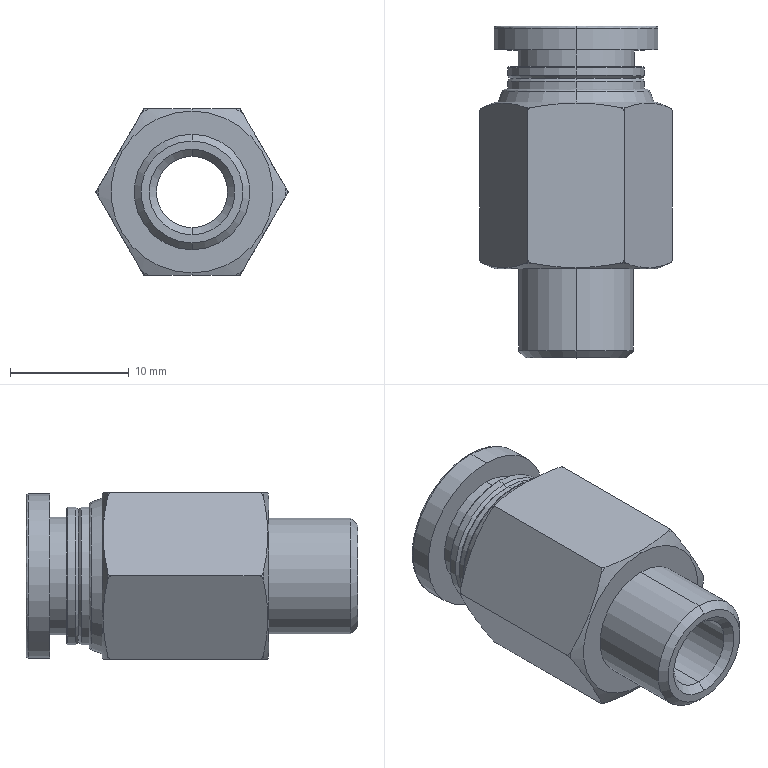Part | STEP file | 11-PC801-V2.011 | 1 solid | 62 faces | box 16.166 x 27.9 x 14 mm | volume 2465 mm3 | spline 18 | cone 16 | cylinder 14 | plane 14 | commonest cylinder face diameters 11.6 x4 6 x2 8 x2 9.728 x2 9.9 x2 13.8 x2